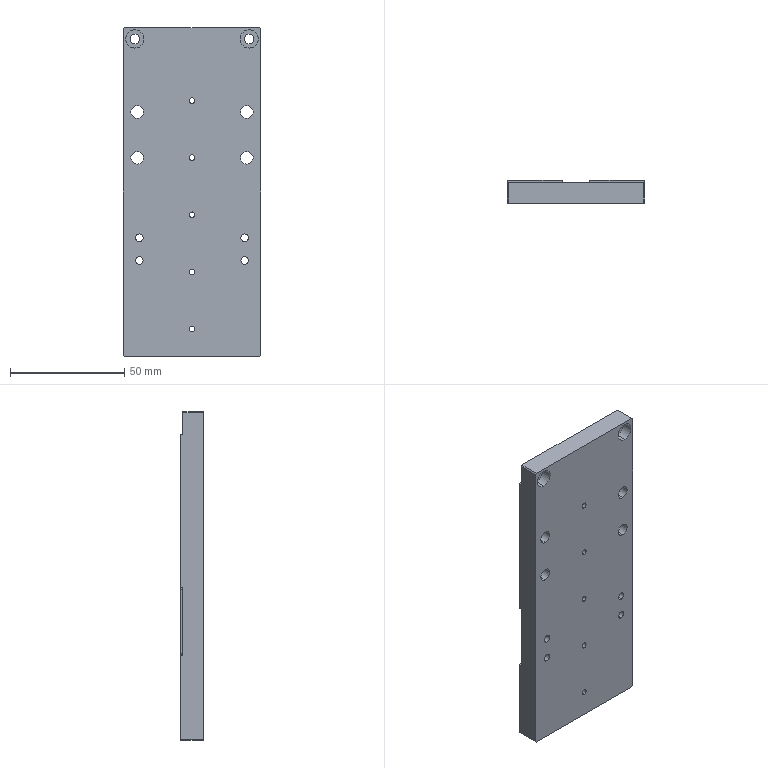Part | STEP file | PN_0053 Mount electronic clip mounting base plate Z-axis | 1 solid | 84 faces | box 60 x 10 x 144 mm | volume 79878 mm3 | cylinder 52 | plane 32 | commonest cylinder face diameters 2.5 x10 3.3 x8 5.5 x8 10 x8 2 x6 4 x4